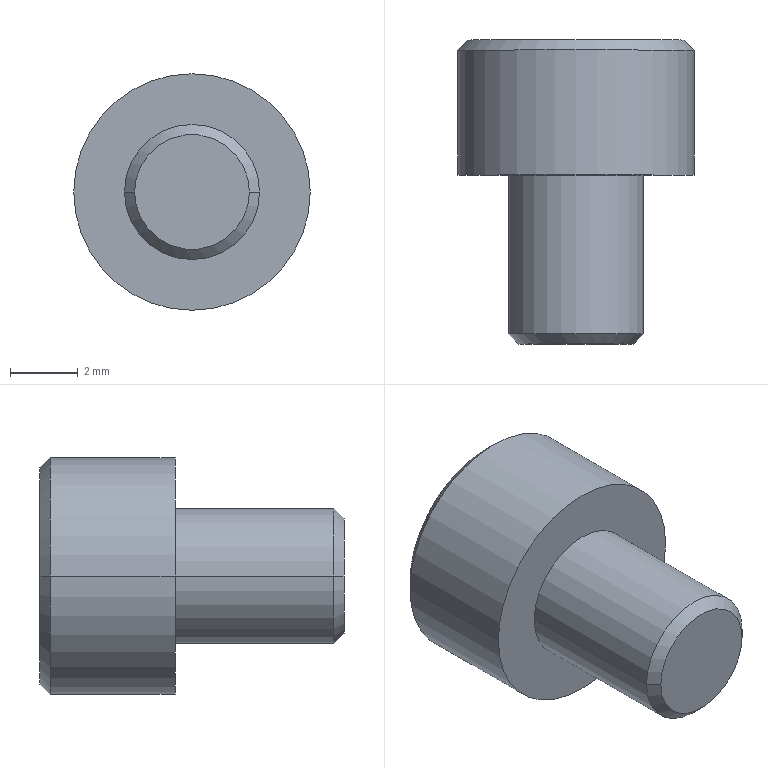Part | NX | 1 solid | 55 faces | box 7 x 9 x 7 mm | volume 197.52 mm3 | plane 45 | cone 6 | cylinder 4 | commonest cylinder face diameters 4 x2 7 x2
STEP:
#1=CARTESIAN_POINT('',(1.7,-5.,0.));
#2=VERTEX_POINT('',#1);
#3=CARTESIAN_POINT('',(-1.7,-5.,0.));
#4=VERTEX_POINT('',#3);
#5=CARTESIAN_POINT('',(0.,-5.,0.));
#6=DIRECTION('',(0.,1.,0.));
#7=DIRECTION('',(-1.,0.,0.));
#8=AXIS2_PLACEMENT_3D('',#5,#6,#7);
#9=CIRCLE('',#8,1.7);
#10=EDGE_CURVE('',#2,#4,#9,.T.);
#11=ORIENTED_EDGE('',*,*,#10,.F.);
#12=CARTESIAN_POINT('',(0.,-5.,0.));
#13=DIRECTION('',(0.,1.,0.));
#14=DIRECTION('',(-1.,0.,0.));
#15=AXIS2_PLACEMENT_3D('',#12,#13,#14);
#16=CIRCLE('',#15,1.7);
#17=EDGE_CURVE('',#4,#2,#16,.T.);
#18=ORIENTED_EDGE('',*,*,#17,.F.);
#19=EDGE_LOOP('',(#11,#18));
#20=FACE_BOUND('',#19,.T.);
#21=CARTESIAN_POINT('',(0.,-5.,0.));
#22=DIRECTION('',(0.,-1.,0.));
#23=DIRECTION('',(0.,0.,-1.));
#24=AXIS2_PLACEMENT_3D('',#21,#22,#23);
#25=PLANE('',#24);
#26=ADVANCED_FACE('',(#20),#25,.T.);
#27=CARTESIAN_POINT('',(-2.,-4.7,0.));
#28=VERTEX_POINT('',#27);
#29=CARTESIAN_POINT('',(2.,-4.7,0.));
#30=VERTEX_POINT('',#29);
#31=CARTESIAN_POINT('',(0.,-4.7,0.));
#32=DIRECTION('',(0.,1.,0.));
#33=DIRECTION('',(-1.,0.,0.));
#34=AXIS2_PLACEMENT_3D('',#31,#32,#33);
#35=CIRCLE('',#34,2.);
#36=EDGE_CURVE('',#28,#30,#35,.T.);
#37=ORIENTED_EDGE('',*,*,#36,.F.);
#38=CARTESIAN_POINT('',(-1.85,-4.85,0.));
#39=DIRECTION('',(-0.7071,0.7071,0.));
#40=VECTOR('',#39,1000.);
#41=LINE('',#38,#40);
#42=EDGE_CURVE('',#28,#4,#41,.F.);
#43=ORIENTED_EDGE('',*,*,#42,.T.);
#44=ORIENTED_EDGE('',*,*,#17,.T.);
#45=CARTESIAN_POINT('',(1.85,-4.85,0.));
#46=DIRECTION('',(0.7071,0.7071,0.));
#47=VECTOR('',#46,1000.);
#48=LINE('',#45,#47);
#49=EDGE_CURVE('',#30,#2,#48,.F.);
#50=ORIENTED_EDGE('',*,*,#49,.F.);
#51=EDGE_LOOP('',(#37,#43,#44,#50));
#52=FACE_BOUND('',#51,.T.);
#53=CARTESIAN_POINT('',(0.,-4.85,0.));
#54=DIRECTION('',(0.,1.,0.));
#55=DIRECTION('',(1.,0.,0.));
#56=AXIS2_PLACEMENT_3D('',#53,#54,#55);
#57=CONICAL_SURFACE('',#56,1.85,0.7854);
#58=ADVANCED_FACE('',(#52),#57,.T.);
#59=CARTESIAN_POINT('',(-2.,0.,0.));
#60=VERTEX_POINT('',#59);
#61=CARTESIAN_POINT('',(2.,0.,0.));
#62=VERTEX_POINT('',#61);
#63=CARTESIAN_POINT('',(0.,0.,0.));
#64=DIRECTION('',(0.,-1.,0.));
#65=DIRECTION('',(1.,0.,0.));
#66=AXIS2_PLACEMENT_3D('',#63,#64,#65);
#67=CIRCLE('',#66,2.);
#68=EDGE_CURVE('',#60,#62,#67,.T.);
#69=ORIENTED_EDGE('',*,*,#68,.T.);
#70=CARTESIAN_POINT('',(2.,4.45,0.));
#71=DIRECTION('',(0.,-1.,0.));
#72=VECTOR('',#71,1000.);
#73=LINE('',#70,#72);
#74=EDGE_CURVE('',#62,#30,#73,.T.);
#75=ORIENTED_EDGE('',*,*,#74,.T.);
#76=CARTESIAN_POINT('',(0.,-4.7,0.));
#77=DIRECTION('',(0.,1.,0.));
#78=DIRECTION('',(-1.,0.,0.));
#79=AXIS2_PLACEMENT_3D('',#76,#77,#78);
#80=CIRCLE('',#79,2.);
#81=EDGE_CURVE('',#30,#28,#80,.T.);
#82=ORIENTED_EDGE('',*,*,#81,.T.);
#83=CARTESIAN_POINT('',(-2.,4.45,0.));
#84=DIRECTION('',(0.,-1.,0.));
#85=VECTOR('',#84,1000.);
#86=LINE('',#83,#85);
#87=EDGE_CURVE('',#60,#28,#86,.T.);
#88=ORIENTED_EDGE('',*,*,#87,.F.);
#89=EDGE_LOOP('',(#69,#75,#82,#88));
#90=FACE_BOUND('',#89,.T.);
#91=CARTESIAN_POINT('',(0.,4.45,0.));
#92=DIRECTION('',(0.,-1.,0.));
#93=DIRECTION('',(-1.,0.,0.));
#94=AXIS2_PLACEMENT_3D('',#91,#92,#93);
#95=CYLINDRICAL_SURFACE('',#94,2.);
#96=ADVANCED_FACE('',(#90),#95,.T.);
#97=CARTESIAN_POINT('',(0.6667,4.,2.274));
#98=VERTEX_POINT('',#97);
#99=CARTESIAN_POINT('',(0.6667,4.,1.87));
#100=VERTEX_POINT('',#99);
#101=CARTESIAN_POINT('',(0.6667,4.,2.274));
#102=DIRECTION('',(0.,0.,-1.));
#103=VECTOR('',#102,1000.);
#104=LINE('',#101,#103);
#105=EDGE_CURVE('',#98,#100,#104,.T.);
#106=ORIENTED_EDGE('',*,*,#105,.F.);
#107=CARTESIAN_POINT('',(0.6667,3.95,2.274));
#108=VERTEX_POINT('',#107);
#109=CARTESIAN_POINT('',(0.6667,3.95,2.274));
#110=DIRECTION('',(0.,1.,0.));
#111=VECTOR('',#110,1000.);
#112=LINE('',#109,#111);
#113=EDGE_CURVE('',#108,#98,#112,.T.);
#114=ORIENTED_EDGE('',*,*,#113,.F.);
#115=CARTESIAN_POINT('',(0.6667,3.95,1.87));
#116=VERTEX_POINT('',#115);
#117=CARTESIAN_POINT('',(0.6667,3.95,2.274));
#118=DIRECTION('',(0.,0.,-1.));
#119=VECTOR('',#118,1000.);
#120=LINE('',#117,#119);
#121=EDGE_CURVE('',#108,#116,#120,.T.);
#122=ORIENTED_EDGE('',*,*,#121,.T.);
#123=CARTESIAN_POINT('',(0.6667,3.95,1.87));
#124=DIRECTION('',(0.,1.,0.));
#125=VECTOR('',#124,1000.);
#126=LINE('',#123,#125);
#127=EDGE_CURVE('',#116,#100,#126,.T.);
#128=ORIENTED_EDGE('',*,*,#127,.T.);
#129=EDGE_LOOP('',(#106,#114,#122,#128));
#130=FACE_BOUND('',#129,.T.);
#131=CARTESIAN_POINT('',(0.6667,4.,1.87));
#132=DIRECTION('',(-1.,0.,0.));
#133=DIRECTION('',(0.,0.,1.));
#134=AXIS2_PLACEMENT_3D('',#131,#132,#133);
#135=PLANE('',#134);
#136=ADVANCED_FACE('',(#130),#135,.F.);
#137=CARTESIAN_POINT('',(0.3125,4.,2.274));
#138=VERTEX_POINT('',#137);
#139=CARTESIAN_POINT('',(0.3125,4.,2.274));
#140=DIRECTION('',(0.659,0.,-0.7522));
#141=VECTOR('',#140,1000.);
#142=LINE('',#139,#141);
#143=EDGE_CURVE('',#138,#100,#142,.T.);
#144=ORIENTED_EDGE('',*,*,#143,.T.);
#145=ORIENTED_EDGE('',*,*,#127,.F.);
#146=CARTESIAN_POINT('',(0.3125,3.95,2.274));
#147=VERTEX_POINT('',#146);
#148=CARTESIAN_POINT('',(0.6667,3.95,1.87));
#149=DIRECTION('',(-0.659,0.,0.7522));
#150=VECTOR('',#149,1000.);
#151=LINE('',#148,#150);
#152=EDGE_CURVE('',#116,#147,#151,.T.);
#153=ORIENTED_EDGE('',*,*,#152,.T.);
#154=CARTESIAN_POINT('',(0.3125,3.95,2.274));
#155=DIRECTION('',(0.,1.,0.));
#156=VECTOR('',#155,1000.);
#157=LINE('',#154,#156);
#158=EDGE_CURVE('',#147,#138,#157,.T.);
#159=ORIENTED_EDGE('',*,*,#158,.T.);
#160=EDGE_LOOP('',(#144,#145,#153,#159));
#161=FACE_BOUND('',#160,.T.);
#162=CARTESIAN_POINT('',(0.3125,4.,2.274));
#163=DIRECTION('',(0.7522,0.,0.659));
#164=DIRECTION('',(0.,-1.,0.));
#165=AXIS2_PLACEMENT_3D('',#162,#163,#164);
#166=PLANE('',#165);
#167=ADVANCED_FACE('',(#161),#166,.F.);
#168=CARTESIAN_POINT('',(-3.5,0.,0.));
#169=VERTEX_POINT('',#168);
#170=CARTESIAN_POINT('',(3.5,0.,0.));
#171=VERTEX_POINT('',#170);
#172=CARTESIAN_POINT('',(0.,0.,0.));
#173=DIRECTION('',(0.,1.,0.));
#174=DIRECTION('',(-1.,0.,0.));
#175=AXIS2_PLACEMENT_3D('',#172,#173,#174);
#176=CIRCLE('',#175,3.5);
#177=EDGE_CURVE('',#169,#171,#176,.T.);
#178=ORIENTED_EDGE('',*,*,#177,.F.);
#179=CARTESIAN_POINT('',(0.,0.,0.));
#180=DIRECTION('',(0.,1.,0.));
#181=DIRECTION('',(-1.,0.,0.));
#182=AXIS2_PLACEMENT_3D('',#179,#180,#181);
#183=CIRCLE('',#182,3.5);
#184=EDGE_CURVE('',#171,#169,#183,.T.);
#185=ORIENTED_EDGE('',*,*,#184,.F.);
#186=EDGE_LOOP('',(#178,#185));
#187=FACE_BOUND('',#186,.T.);
#188=ORIENTED_EDGE('',*,*,#68,.F.);
#189=CARTESIAN_POINT('',(0.,0.,0.));
#190=DIRECTION('',(0.,-1.,0.));
#191=DIRECTION('',(1.,0.,0.));
#192=AXIS2_PLACEMENT_3D('',#189,#190,#191);
#193=CIRCLE('',#192,2.);
#194=EDGE_CURVE('',#62,#60,#193,.T.);
#195=ORIENTED_EDGE('',*,*,#194,.F.);
#196=EDGE_LOOP('',(#188,#195));
#197=FACE_BOUND('',#196,.T.);
#198=CARTESIAN_POINT('',(0.,0.,0.));
#199=DIRECTION('',(0.,-1.,0.));
#200=DIRECTION('',(0.,0.,-1.));
#201=AXIS2_PLACEMENT_3D('',#198,#199,#200);
#202=PLANE('',#201);
#203=ADVANCED_FACE('',(#187,#197),#202,.T.);
#204=ORIENTED_EDGE('',*,*,#177,.T.);
#205=CARTESIAN_POINT('',(3.5,3.7,0.));
#206=VERTEX_POINT('',#205);
#207=CARTESIAN_POINT('',(3.5,4.45,0.));
#208=DIRECTION('',(0.,-1.,0.));
#209=VECTOR('',#208,1000.);
#210=LINE('',#207,#209);
#211=EDGE_CURVE('',#206,#171,#210,.T.);
#212=ORIENTED_EDGE('',*,*,#211,.F.);
#213=CARTESIAN_POINT('',(-3.5,3.7,0.));
#214=VERTEX_POINT('',#213);
#215=CARTESIAN_POINT('',(0.,3.7,0.));
#216=DIRECTION('',(0.,-1.,0.));
#217=DIRECTION('',(1.,0.,0.));
#218=AXIS2_PLACEMENT_3D('',#215,#216,#217);
#219=CIRCLE('',#218,3.5);
#220=EDGE_CURVE('',#206,#214,#219,.T.);
#221=ORIENTED_EDGE('',*,*,#220,.T.);
#222=CARTESIAN_POINT('',(-3.5,4.45,0.));
#223=DIRECTION('',(0.,-1.,0.));
#224=VECTOR('',#223,1000.);
#225=LINE('',#222,#224);
#226=EDGE_CURVE('',#214,#169,#225,.T.);
#227=ORIENTED_EDGE('',*,*,#226,.T.);
#228=EDGE_LOOP('',(#204,#212,#221,#227));
#229=FACE_BOUND('',#228,.T.);
#230=CARTESIAN_POINT('',(0.,4.45,0.));
#231=DIRECTION('',(0.,-1.,0.));
#232=DIRECTION('',(-1.,0.,0.));
#233=AXIS2_PLACEMENT_3D('',#230,#231,#232);
#234=CYLINDRICAL_SURFACE('',#233,3.5);
#235=ADVANCED_FACE('',(#229),#234,.T.);
#236=CARTESIAN_POINT('',(0.1667,3.95,2.274));
#237=VERTEX_POINT('',#236);
#238=CARTESIAN_POINT('',(0.6667,3.95,1.7));
#239=VERTEX_POINT('',#238);
#240=CARTESIAN_POINT('',(0.1667,3.95,2.274));
#241=DIRECTION('',(0.6565,0.,-0.7543));
#242=VECTOR('',#241,1000.);
#243=LINE('',#240,#242);
#244=EDGE_CURVE('',#237,#239,#243,.T.);
#245=ORIENTED_EDGE('',*,*,#244,.F.);
#246=CARTESIAN_POINT('',(0.1667,3.95,2.402));
#247=VERTEX_POINT('',#246);
#248=CARTESIAN_POINT('',(0.1667,3.95,2.402));
#249=DIRECTION('',(0.,0.,-1.));
#250=VECTOR('',#249,1000.);
#251=LINE('',#248,#250);
#252=EDGE_CURVE('',#247,#237,#251,.T.);
#253=ORIENTED_EDGE('',*,*,#252,.F.);
#254=CARTESIAN_POINT('',(0.6667,3.95,2.402));
#255=VERTEX_POINT('',#254);
#256=CARTESIAN_POINT('',(0.6667,3.95,2.402));
#257=DIRECTION('',(-1.,0.,0.));
#258=VECTOR('',#257,1000.);
#259=LINE('',#256,#258);
#260=EDGE_CURVE('',#255,#247,#259,.T.);
#261=ORIENTED_EDGE('',*,*,#260,.F.);
#262=CARTESIAN_POINT('',(0.6667,3.95,2.7));
#263=VERTEX_POINT('',#262);
#264=CARTESIAN_POINT('',(0.6667,3.95,2.7));
#265=DIRECTION('',(0.,0.,-1.));
#266=VECTOR('',#265,1000.);
#267=LINE('',#264,#266);
#268=EDGE_CURVE('',#263,#255,#267,.T.);
#269=ORIENTED_EDGE('',*,*,#268,.F.);
#270=CARTESIAN_POINT('',(0.7917,3.95,2.7));
#271=VERTEX_POINT('',#270);
#272=CARTESIAN_POINT('',(0.7917,3.95,2.7));
#273=DIRECTION('',(-1.,0.,0.));
#274=VECTOR('',#273,1000.);
#275=LINE('',#272,#274);
#276=EDGE_CURVE('',#271,#263,#275,.T.);
#277=ORIENTED_EDGE('',*,*,#276,.F.);
#278=CARTESIAN_POINT('',(0.7917,3.95,2.402));
#279=VERTEX_POINT('',#278);
#280=CARTESIAN_POINT('',(0.7917,3.95,2.402));
#281=DIRECTION('',(0.,0.,1.));
#282=VECTOR('',#281,1000.);
#283=LINE('',#280,#282);
#284=EDGE_CURVE('',#279,#271,#283,.T.);
#285=ORIENTED_EDGE('',*,*,#284,.F.);
#286=CARTESIAN_POINT('',(1.,3.95,2.402));
#287=VERTEX_POINT('',#286);
#288=CARTESIAN_POINT('',(1.,3.95,2.402));
#289=DIRECTION('',(-1.,0.,0.));
#290=VECTOR('',#289,1000.);
#291=LINE('',#288,#290);
#292=EDGE_CURVE('',#287,#279,#291,.T.);
#293=ORIENTED_EDGE('',*,*,#292,.F.);
#294=CARTESIAN_POINT('',(1.,3.95,2.274));
#295=VERTEX_POINT('',#294);
#296=CARTESIAN_POINT('',(1.,3.95,2.274));
#297=DIRECTION('',(0.,0.,1.));
#298=VECTOR('',#297,1000.);
#299=LINE('',#296,#298);
#300=EDGE_CURVE('',#295,#287,#299,.T.);
#301=ORIENTED_EDGE('',*,*,#300,.F.);
#302=CARTESIAN_POINT('',(0.7917,3.95,2.274));
#303=VERTEX_POINT('',#302);
#304=CARTESIAN_POINT('',(0.7917,3.95,2.274));
#305=DIRECTION('',(1.,0.,0.));
#306=VECTOR('',#305,1000.);
#307=LINE('',#304,#306);
#308=EDGE_CURVE('',#303,#295,#307,.T.);
#309=ORIENTED_EDGE('',*,*,#308,.F.);
#310=CARTESIAN_POINT('',(0.7917,3.95,1.7));
#311=VERTEX_POINT('',#310);
#312=CARTESIAN_POINT('',(0.7917,3.95,1.7));
#313=DIRECTION('',(0.,0.,1.));
#314=VECTOR('',#313,1000.);
#315=LINE('',#312,#314);
#316=EDGE_CURVE('',#311,#303,#315,.T.);
#317=ORIENTED_EDGE('',*,*,#316,.F.);
#318=CARTESIAN_POINT('',(0.6667,3.95,1.7));
#319=DIRECTION('',(1.,0.,0.));
#320=VECTOR('',#319,1000.);
#321=LINE('',#318,#320);
#322=EDGE_CURVE('',#239,#311,#321,.T.);
#323=ORIENTED_EDGE('',*,*,#322,.F.);
#324=EDGE_LOOP('',(#245,#253,#261,#269,#277,#285,#293,#301,#309,#317,#323));
#325=FACE_BOUND('',#324,.T.);
#326=ORIENTED_EDGE('',*,*,#152,.F.);
#327=ORIENTED_EDGE('',*,*,#121,.F.);
#328=CARTESIAN_POINT('',(0.3125,3.95,2.274));
#329=DIRECTION('',(1.,0.,0.));
#330=VECTOR('',#329,1000.);
#331=LINE('',#328,#330);
#332=EDGE_CURVE('',#147,#108,#331,.T.);
#333=ORIENTED_EDGE('',*,*,#332,.F.);
#334=EDGE_LOOP('',(#326,#327,#333));
#335=FACE_BOUND('',#334,.T.);
#336=CARTESIAN_POINT('',(0.,3.95,0.));
#337=DIRECTION('',(0.,1.,0.));
#338=DIRECTION('',(1.,0.,0.));
#339=AXIS2_PLACEMENT_3D('',#336,#337,#338);
#340=PLANE('',#339);
#341=ADVANCED_FACE('',(#325,#335),#340,.T.);
#342=CARTESIAN_POINT('',(0.,3.7,0.));
#343=DIRECTION('',(0.,-1.,0.));
#344=DIRECTION('',(1.,0.,0.));
#345=AXIS2_PLACEMENT_3D('',#342,#343,#344);
#346=CIRCLE('',#345,3.5);
#347=EDGE_CURVE('',#214,#206,#346,.T.);
#348=ORIENTED_EDGE('',*,*,#347,.F.);
#349=CARTESIAN_POINT('',(-3.2,4.,0.));
#350=VERTEX_POINT('',#349);
#351=CARTESIAN_POINT('',(-3.35,3.85,0.));
#352=DIRECTION('',(-0.7071,-0.7071,0.));
#353=VECTOR('',#352,1000.);
#354=LINE('',#351,#353);
#355=EDGE_CURVE('',#214,#350,#354,.F.);
#356=ORIENTED_EDGE('',*,*,#355,.T.);
#357=CARTESIAN_POINT('',(3.2,4.,0.));
#358=VERTEX_POINT('',#357);
#359=CARTESIAN_POINT('',(0.,4.,0.));
#360=DIRECTION('',(0.,-1.,0.));
#361=DIRECTION('',(-1.,0.,0.));
#362=AXIS2_PLACEMENT_3D('',#359,#360,#361);
#363=CIRCLE('',#362,3.2);
#364=EDGE_CURVE('',#350,#358,#363,.T.);
#365=ORIENTED_EDGE('',*,*,#364,.T.);
#366=CARTESIAN_POINT('',(3.35,3.85,0.));
#367=DIRECTION('',(0.7071,-0.7071,0.));
#368=VECTOR('',#367,1000.);
#369=LINE('',#366,#368);
#370=EDGE_CURVE('',#206,#358,#369,.F.);
#371=ORIENTED_EDGE('',*,*,#370,.F.);
#372=EDGE_LOOP('',(#348,#356,#365,#371));
#373=FACE_BOUND('',#372,.T.);
#374=CARTESIAN_POINT('',(0.,3.85,0.));
#375=DIRECTION('',(0.,-1.,0.));
#376=DIRECTION('',(-1.,0.,0.));
#377=AXIS2_PLACEMENT_3D('',#374,#375,#376);
#378=CONICAL_SURFACE('',#377,3.35,0.7854);
#379=ADVANCED_FACE('',(#373),#378,.T.);
#380=ORIENTED_EDGE('',*,*,#364,.F.);
#381=CARTESIAN_POINT('',(0.,4.,0.));
#382=DIRECTION('',(0.,-1.,0.));
#383=DIRECTION('',(-1.,0.,0.));
#384=AXIS2_PLACEMENT_3D('',#381,#382,#383);
#385=CIRCLE('',#384,3.2);
#386=EDGE_CURVE('',#358,#350,#385,.T.);
#387=ORIENTED_EDGE('',*,*,#386,.F.);
#388=EDGE_LOOP('',(#380,#387));
#389=FACE_BOUND('',#388,.T.);
#390=CARTESIAN_POINT('',(-0.125,4.,2.7));
#391=VERTEX_POINT('',#390);
#392=CARTESIAN_POINT('',(-0.125,4.,1.913));
#393=VERTEX_POINT('',#392);
#394=CARTESIAN_POINT('',(-0.125,4.,2.7));
#395=DIRECTION('',(0.,0.,-1.));
#396=VECTOR('',#395,1000.);
#397=LINE('',#394,#396);
#398=EDGE_CURVE('',#391,#393,#397,.T.);
#399=ORIENTED_EDGE('',*,*,#398,.T.);
#400=CARTESIAN_POINT('',(-0.4167,4.,2.7));
#401=VERTEX_POINT('',#400);
#402=CARTESIAN_POINT('',(-0.4167,4.,2.7));
#403=DIRECTION('',(0.3474,0.,-0.9377));
#404=VECTOR('',#403,1000.);
#405=LINE('',#402,#404);
#406=EDGE_CURVE('',#401,#393,#405,.T.);
#407=ORIENTED_EDGE('',*,*,#406,.F.);
#408=CARTESIAN_POINT('',(-0.5833,4.,2.7));
#409=VERTEX_POINT('',#408);
#410=CARTESIAN_POINT('',(-0.4167,4.,2.7));
#411=DIRECTION('',(-1.,0.,0.));
#412=VECTOR('',#411,1000.);
#413=LINE('',#410,#412);
#414=EDGE_CURVE('',#401,#409,#413,.T.);
#415=ORIENTED_EDGE('',*,*,#414,.T.);
#416=CARTESIAN_POINT('',(-0.875,4.,1.913));
#417=VERTEX_POINT('',#416);
#418=CARTESIAN_POINT('',(-0.875,4.,1.913));
#419=DIRECTION('',(0.3474,0.,0.9377));
#420=VECTOR('',#419,1000.);
#421=LINE('',#418,#420);
#422=EDGE_CURVE('',#417,#409,#421,.T.);
#423=ORIENTED_EDGE('',*,*,#422,.F.);
#424=CARTESIAN_POINT('',(-0.875,4.,2.7));
#425=VERTEX_POINT('',#424);
#426=CARTESIAN_POINT('',(-0.875,4.,1.913));
#427=DIRECTION('',(0.,0.,1.));
#428=VECTOR('',#427,1000.);
#429=LINE('',#426,#428);
#430=EDGE_CURVE('',#417,#425,#429,.T.);
#431=ORIENTED_EDGE('',*,*,#430,.T.);
#432=CARTESIAN_POINT('',(-1.,4.,2.7));
#433=VERTEX_POINT('',#432);
#434=CARTESIAN_POINT('',(-0.875,4.,2.7));
#435=DIRECTION('',(-1.,0.,0.));
#436=VECTOR('',#435,1000.);
#437=LINE('',#434,#436);
#438=EDGE_CURVE('',#425,#433,#437,.T.);
#439=ORIENTED_EDGE('',*,*,#438,.T.);
#440=CARTESIAN_POINT('',(-1.,4.,1.7));
#441=VERTEX_POINT('',#440);
#442=CARTESIAN_POINT('',(-1.,4.,2.7));
#443=DIRECTION('',(0.,0.,-1.));
#444=VECTOR('',#443,1000.);
#445=LINE('',#442,#444);
#446=EDGE_CURVE('',#433,#441,#445,.T.);
#447=ORIENTED_EDGE('',*,*,#446,.T.);
#448=CARTESIAN_POINT('',(-0.8125,4.,1.7));
#449=VERTEX_POINT('',#448);
#450=CARTESIAN_POINT('',(-1.,4.,1.7));
#451=DIRECTION('',(1.,0.,0.));
#452=VECTOR('',#451,1000.);
#453=LINE('',#450,#452);
#454=EDGE_CURVE('',#441,#449,#453,.T.);
#455=ORIENTED_EDGE('',*,*,#454,.T.);
#456=CARTESIAN_POINT('',(-0.5,4.,2.594));
#457=VERTEX_POINT('',#456);
#458=CARTESIAN_POINT('',(-0.5,4.,2.594));
#459=DIRECTION('',(-0.3301,0.,-0.9439));
#460=VECTOR('',#459,1000.);
#461=LINE('',#458,#460);
#462=EDGE_CURVE('',#457,#449,#461,.T.);
#463=ORIENTED_EDGE('',*,*,#462,.F.);
#464=CARTESIAN_POINT('',(-0.1875,4.,1.7));
#465=VERTEX_POINT('',#464);
#466=CARTESIAN_POINT('',(-0.1875,4.,1.7));
#467=DIRECTION('',(-0.3301,0.,0.9439));
#468=VECTOR('',#467,1000.);
#469=LINE('',#466,#468);
#470=EDGE_CURVE('',#465,#457,#469,.T.);
#471=ORIENTED_EDGE('',*,*,#470,.F.);
#472=CARTESIAN_POINT('',(-0.05551,4.,1.7));
#473=VERTEX_POINT('',#472);
#474=CARTESIAN_POINT('',(-0.1875,4.,1.7));
#475=DIRECTION('',(1.,0.,0.));
#476=VECTOR('',#475,1000.);
#477=LINE('',#474,#476);
#478=EDGE_CURVE('',#465,#473,#477,.T.);
#479=ORIENTED_EDGE('',*,*,#478,.T.);
#480=CARTESIAN_POINT('',(-1.5,4.,0.866));
#481=VERTEX_POINT('',#480);
#482=CARTESIAN_POINT('',(-1.5,4.,0.866));
#483=DIRECTION('',(0.866,0.,0.5));
#484=VECTOR('',#483,1000.);
#485=LINE('',#482,#484);
#486=EDGE_CURVE('',#481,#473,#485,.T.);
#487=ORIENTED_EDGE('',*,*,#486,.F.);
#488=CARTESIAN_POINT('',(-1.5,4.,-0.866));
#489=VERTEX_POINT('',#488);
#490=CARTESIAN_POINT('',(-1.5,4.,0.866));
#491=DIRECTION('',(0.,0.,-1.));
#492=VECTOR('',#491,1000.);
#493=LINE('',#490,#492);
#494=EDGE_CURVE('',#481,#489,#493,.T.);
#495=ORIENTED_EDGE('',*,*,#494,.T.);
#496=CARTESIAN_POINT('',(0.,4.,-1.732));
#497=VERTEX_POINT('',#496);
#498=CARTESIAN_POINT('',(0.,4.,-1.732));
#499=DIRECTION('',(-0.866,0.,0.5));
#500=VECTOR('',#499,1000.);
#501=LINE('',#498,#500);
#502=EDGE_CURVE('',#497,#489,#501,.T.);
#503=ORIENTED_EDGE('',*,*,#502,.F.);
#504=CARTESIAN_POINT('',(1.5,4.,-0.866));
#505=VERTEX_POINT('',#504);
#506=CARTESIAN_POINT('',(1.5,4.,-0.866));
#507=DIRECTION('',(-0.866,0.,-0.5));
#508=VECTOR('',#507,1000.);
#509=LINE('',#506,#508);
#510=EDGE_CURVE('',#505,#497,#509,.T.);
#511=ORIENTED_EDGE('',*,*,#510,.F.);
#512=CARTESIAN_POINT('',(1.5,4.,0.866));
#513=VERTEX_POINT('',#512);
#514=CARTESIAN_POINT('',(1.5,4.,-0.866));
#515=DIRECTION('',(0.,0.,1.));
#516=VECTOR('',#515,1000.);
#517=LINE('',#514,#516);
#518=EDGE_CURVE('',#505,#513,#517,.T.);
#519=ORIENTED_EDGE('',*,*,#518,.T.);
#520=CARTESIAN_POINT('',(0.,4.,1.732));
#521=VERTEX_POINT('',#520);
#522=CARTESIAN_POINT('',(0.,4.,1.732));
#523=DIRECTION('',(0.866,0.,-0.5));
#524=VECTOR('',#523,1000.);
#525=LINE('',#522,#524);
#526=EDGE_CURVE('',#521,#513,#525,.T.);
#527=ORIENTED_EDGE('',*,*,#526,.F.);
#528=CARTESIAN_POINT('',(0.,4.,2.7));
#529=VERTEX_POINT('',#528);
#530=CARTESIAN_POINT('',(0.,4.,1.732));
#531=DIRECTION('',(0.,0.,1.));
#532=VECTOR('',#531,1000.);
#533=LINE('',#530,#532);
#534=EDGE_CURVE('',#521,#529,#533,.T.);
#535=ORIENTED_EDGE('',*,*,#534,.T.);
#536=CARTESIAN_POINT('',(0.,4.,2.7));
#537=DIRECTION('',(-1.,0.,0.));
#538=VECTOR('',#537,1000.);
#539=LINE('',#536,#538);
#540=EDGE_CURVE('',#529,#391,#539,.T.);
#541=ORIENTED_EDGE('',*,*,#540,.T.);
#542=EDGE_LOOP('',(#399,#407,#415,#423,#431,#439,#447,#455,#463,#471,#479,#487,#495,#503,#511,#519,#527,#535,#541));
#543=FACE_BOUND('',#542,.T.);
#544=CARTESIAN_POINT('',(0.6667,4.,1.7));
#545=VERTEX_POINT('',#544);
#546=CARTESIAN_POINT('',(0.1667,4.,2.274));
#547=VERTEX_POINT('',#546);
#548=CARTESIAN_POINT('',(0.6667,4.,1.7));
#549=DIRECTION('',(-0.6565,0.,0.7543));
#550=VECTOR('',#549,1000.);
#551=LINE('',#548,#550);
#552=EDGE_CURVE('',#545,#547,#551,.T.);
#553=ORIENTED_EDGE('',*,*,#552,.F.);
#554=CARTESIAN_POINT('',(0.7917,4.,1.7));
#555=VERTEX_POINT('',#554);
#556=CARTESIAN_POINT('',(0.6667,4.,1.7));
#557=DIRECTION('',(1.,0.,0.));
#558=VECTOR('',#557,1000.);
#559=LINE('',#556,#558);
#560=EDGE_CURVE('',#545,#555,#559,.T.);
#561=ORIENTED_EDGE('',*,*,#560,.T.);
#562=CARTESIAN_POINT('',(0.7917,4.,2.274));
#563=VERTEX_POINT('',#562);
#564=CARTESIAN_POINT('',(0.7917,4.,1.7));
#565=DIRECTION('',(0.,0.,1.));
#566=VECTOR('',#565,1000.);
#567=LINE('',#564,#566);
#568=EDGE_CURVE('',#555,#563,#567,.T.);
#569=ORIENTED_EDGE('',*,*,#568,.T.);
#570=CARTESIAN_POINT('',(1.,4.,2.274));
#571=VERTEX_POINT('',#570);
#572=CARTESIAN_POINT('',(0.7917,4.,2.274));
#573=DIRECTION('',(1.,0.,0.));
#574=VECTOR('',#573,1000.);
#575=LINE('',#572,#574);
#576=EDGE_CURVE('',#563,#571,#575,.T.);
#577=ORIENTED_EDGE('',*,*,#576,.T.);
#578=CARTESIAN_POINT('',(1.,4.,2.402));
#579=VERTEX_POINT('',#578);
#580=CARTESIAN_POINT('',(1.,4.,2.274));
#581=DIRECTION('',(0.,0.,1.));
#582=VECTOR('',#581,1000.);
#583=LINE('',#580,#582);
#584=EDGE_CURVE('',#571,#579,#583,.T.);
#585=ORIENTED_EDGE('',*,*,#584,.T.);
#586=CARTESIAN_POINT('',(0.7917,4.,2.402));
#587=VERTEX_POINT('',#586);
#588=CARTESIAN_POINT('',(1.,4.,2.402));
#589=DIRECTION('',(-1.,0.,0.));
#590=VECTOR('',#589,1000.);
#591=LINE('',#588,#590);
#592=EDGE_CURVE('',#579,#587,#591,.T.);
#593=ORIENTED_EDGE('',*,*,#592,.T.);
#594=CARTESIAN_POINT('',(0.7917,4.,2.7));
#595=VERTEX_POINT('',#594);
#596=CARTESIAN_POINT('',(0.7917,4.,2.402));
#597=DIRECTION('',(0.,0.,1.));
#598=VECTOR('',#597,1000.);
#599=LINE('',#596,#598);
#600=EDGE_CURVE('',#587,#595,#599,.T.);
#601=ORIENTED_EDGE('',*,*,#600,.T.);
#602=CARTESIAN_POINT('',(0.6667,4.,2.7));
#603=VERTEX_POINT('',#602);
#604=CARTESIAN_POINT('',(0.7917,4.,2.7));
#605=DIRECTION('',(-1.,0.,0.));
#606=VECTOR('',#605,1000.);
#607=LINE('',#604,#606);
#608=EDGE_CURVE('',#595,#603,#607,.T.);
#609=ORIENTED_EDGE('',*,*,#608,.T.);
#610=CARTESIAN_POINT('',(0.6667,4.,2.402));
#611=VERTEX_POINT('',#610);
#612=CARTESIAN_POINT('',(0.6667,4.,2.7));
#613=DIRECTION('',(0.,0.,-1.));
#614=VECTOR('',#613,1000.);
#615=LINE('',#612,#614);
#616=EDGE_CURVE('',#603,#611,#615,.T.);
#617=ORIENTED_EDGE('',*,*,#616,.T.);
#618=CARTESIAN_POINT('',(0.1667,4.,2.402));
#619=VERTEX_POINT('',#618);
#620=CARTESIAN_POINT('',(0.6667,4.,2.402));
#621=DIRECTION('',(-1.,0.,0.));
#622=VECTOR('',#621,1000.);
#623=LINE('',#620,#622);
#624=EDGE_CURVE('',#611,#619,#623,.T.);
#625=ORIENTED_EDGE('',*,*,#624,.T.);
#626=CARTESIAN_POINT('',(0.1667,4.,2.402));
#627=DIRECTION('',(0.,0.,-1.));
#628=VECTOR('',#627,1000.);
#629=LINE('',#626,#628);
#630=EDGE_CURVE('',#619,#547,#629,.T.);
#631=ORIENTED_EDGE('',*,*,#630,.T.);
#632=EDGE_LOOP('',(#553,#561,#569,#577,#585,#593,#601,#609,#617,#625,#631));
#633=FACE_BOUND('',#632,.T.);
#634=CARTESIAN_POINT('',(0.,4.,0.));
#635=DIRECTION('',(0.,-1.,0.));
#636=DIRECTION('',(0.,0.,-1.));
#637=AXIS2_PLACEMENT_3D('',#634,#635,#636);
#638=PLANE('',#637);
#639=ADVANCED_FACE('',(#389,#543,#633),#638,.F.);
#640=ORIENTED_EDGE('',*,*,#143,.F.);
#641=CARTESIAN_POINT('',(0.3125,4.,2.274));
#642=DIRECTION('',(1.,0.,0.));
#643=VECTOR('',#642,1000.);
#644=LINE('',#641,#643);
#645=EDGE_CURVE('',#138,#98,#644,.T.);
#646=ORIENTED_EDGE('',*,*,#645,.T.);
#647=ORIENTED_EDGE('',*,*,#105,.T.);
#648=EDGE_LOOP('',(#640,#646,#647));
#649=FACE_BOUND('',#648,.T.);
#650=CARTESIAN_POINT('',(0.,4.,0.));
#651=DIRECTION('',(0.,-1.,0.));
#652=DIRECTION('',(0.,0.,-1.));
#653=AXIS2_PLACEMENT_3D('',#650,#651,#652);
#654=PLANE('',#653);
#655=ADVANCED_FACE('',(#649),#654,.F.);
#656=ORIENTED_EDGE('',*,*,#398,.F.);
#657=CARTESIAN_POINT('',(-0.125,3.95,2.7));
#658=VERTEX_POINT('',#657);
#659=CARTESIAN_POINT('',(-0.125,3.95,2.7));
#660=DIRECTION('',(0.,1.,0.));
#661=VECTOR('',#660,1000.);
#662=LINE('',#659,#661);
#663=EDGE_CURVE('',#658,#391,#662,.T.);
#664=ORIENTED_EDGE('',*,*,#663,.F.);
#665=CARTESIAN_POINT('',(-0.125,3.95,1.913));
#666=VERTEX_POINT('',#665);
#667=CARTESIAN_POINT('',(-0.125,3.95,2.7));
#668=DIRECTION('',(0.,0.,-1.));
#669=VECTOR('',#668,1000.);
#670=LINE('',#667,#669);
#671=EDGE_CURVE('',#658,#666,#670,.T.);
#672=ORIENTED_EDGE('',*,*,#671,.T.);
#673=CARTESIAN_POINT('',(-0.125,3.95,1.913));
#674=DIRECTION('',(0.,1.,0.));
#675=VECTOR('',#674,1000.);
#676=LINE('',#673,#675);
#677=EDGE_CURVE('',#666,#393,#676,.T.);
#678=ORIENTED_EDGE('',*,*,#677,.T.);
#679=EDGE_LOOP('',(#656,#664,#672,#678));
#680=FACE_BOUND('',#679,.T.);
#681=CARTESIAN_POINT('',(-0.125,4.,1.913));
#682=DIRECTION('',(-1.,0.,0.));
#683=DIRECTION('',(0.,0.,1.));
#684=AXIS2_PLACEMENT_3D('',#681,#682,#683);
#685=PLANE('',#684);
#686=ADVANCED_FACE('',(#680),#685,.F.);
#687=ORIENTED_EDGE('',*,*,#406,.T.);
#688=ORIENTED_EDGE('',*,*,#677,.F.);
#689=CARTESIAN_POINT('',(-0.4167,3.95,2.7));
#690=VERTEX_POINT('',#689);
#691=CARTESIAN_POINT('',(-0.125,3.95,1.913));
#692=DIRECTION('',(-0.3474,0.,0.9377));
#693=VECTOR('',#692,1000.);
#694=LINE('',#691,#693);
#695=EDGE_CURVE('',#666,#690,#694,.T.);
#696=ORIENTED_EDGE('',*,*,#695,.T.);
#697=CARTESIAN_POINT('',(-0.4167,3.95,2.7));
#698=DIRECTION('',(0.,1.,0.));
#699=VECTOR('',#698,1000.);
#700=LINE('',#697,#699);
#701=EDGE_CURVE('',#690,#401,#700,.T.);
#702=ORIENTED_EDGE('',*,*,#701,.T.);
#703=EDGE_LOOP('',(#687,#688,#696,#702));
#704=FACE_BOUND('',#703,.T.);
#705=CARTESIAN_POINT('',(-0.4167,4.,2.7));
#706=DIRECTION('',(0.9377,0.,0.3474));
#707=DIRECTION('',(0.,-1.,0.));
#708=AXIS2_PLACEMENT_3D('',#705,#706,#707);
#709=PLANE('',#708);
#710=ADVANCED_FACE('',(#704),#709,.F.);
#711=ORIENTED_EDGE('',*,*,#414,.F.);
#712=ORIENTED_EDGE('',*,*,#701,.F.);
#713=CARTESIAN_POINT('',(-0.5833,3.95,2.7));
#714=VERTEX_POINT('',#713);
#715=CARTESIAN_POINT('',(-0.4167,3.95,2.7));
#716=DIRECTION('',(-1.,0.,0.));
#717=VECTOR('',#716,1000.);
#718=LINE('',#715,#717);
#719=EDGE_CURVE('',#690,#714,#718,.T.);
#720=ORIENTED_EDGE('',*,*,#719,.T.);
#721=CARTESIAN_POINT('',(-0.5833,3.95,2.7));
#722=DIRECTION('',(0.,1.,0.));
#723=VECTOR('',#722,1000.);
#724=LINE('',#721,#723);
#725=EDGE_CURVE('',#714,#409,#724,.T.);
#726=ORIENTED_EDGE('',*,*,#725,.T.);
#727=EDGE_LOOP('',(#711,#712,#720,#726));
#728=FACE_BOUND('',#727,.T.);
#729=CARTESIAN_POINT('',(-0.5833,4.,2.7));
#730=DIRECTION('',(0.,0.,1.));
#731=DIRECTION('',(1.,0.,0.));
#732=AXIS2_PLACEMENT_3D('',#729,#730,#731);
#733=PLANE('',#732);
#734=ADVANCED_FACE('',(#728),#733,.F.);
#735=ORIENTED_EDGE('',*,*,#422,.T.);
#736=ORIENTED_EDGE('',*,*,#725,.F.);
#737=CARTESIAN_POINT('',(-0.875,3.95,1.913));
#738=VERTEX_POINT('',#737);
#739=CARTESIAN_POINT('',(-0.5833,3.95,2.7));
#740=DIRECTION('',(-0.3474,0.,-0.9377));
#741=VECTOR('',#740,1000.);
#742=LINE('',#739,#741);
#743=EDGE_CURVE('',#714,#738,#742,.T.);
#744=ORIENTED_EDGE('',*,*,#743,.T.);
#745=CARTESIAN_POINT('',(-0.875,3.95,1.913));
#746=DIRECTION('',(0.,1.,0.));
#747=VECTOR('',#746,1000.);
#748=LINE('',#745,#747);
#749=EDGE_CURVE('',#738,#417,#748,.T.);
#750=ORIENTED_EDGE('',*,*,#749,.T.);
#751=EDGE_LOOP('',(#735,#736,#744,#750));
#752=FACE_BOUND('',#751,.T.);
#753=CARTESIAN_POINT('',(-0.875,4.,1.913));
#754=DIRECTION('',(-0.9377,0.,0.3474));
#755=DIRECTION('',(0.,1.,0.));
#756=AXIS2_PLACEMENT_3D('',#753,#754,#755);
#757=PLANE('',#756);
#758=ADVANCED_FACE('',(#752),#757,.F.);
#759=ORIENTED_EDGE('',*,*,#430,.F.);
#760=ORIENTED_EDGE('',*,*,#749,.F.);
#761=CARTESIAN_POINT('',(-0.875,3.95,2.7));
#762=VERTEX_POINT('',#761);
#763=CARTESIAN_POINT('',(-0.875,3.95,1.913));
#764=DIRECTION('',(0.,0.,1.));
#765=VECTOR('',#764,1000.);
#766=LINE('',#763,#765);
#767=EDGE_CURVE('',#738,#762,#766,.T.);
#768=ORIENTED_EDGE('',*,*,#767,.T.);
#769=CARTESIAN_POINT('',(-0.875,3.95,2.7));
#770=DIRECTION('',(0.,1.,0.));
#771=VECTOR('',#770,1000.);
#772=LINE('',#769,#771);
#773=EDGE_CURVE('',#762,#425,#772,.T.);
#774=ORIENTED_EDGE('',*,*,#773,.T.);
#775=EDGE_LOOP('',(#759,#760,#768,#774));
#776=FACE_BOUND('',#775,.T.);
#777=CARTESIAN_POINT('',(-0.875,4.,2.7));
#778=DIRECTION('',(1.,0.,0.));
#779=DIRECTION('',(0.,1.,0.));
#780=AXIS2_PLACEMENT_3D('',#777,#778,#779);
#781=PLANE('',#780);
#782=ADVANCED_FACE('',(#776),#781,.F.);
#783=ORIENTED_EDGE('',*,*,#438,.F.);
#784=ORIENTED_EDGE('',*,*,#773,.F.);
#785=CARTESIAN_POINT('',(-1.,3.95,2.7));
#786=VERTEX_POINT('',#785);
#787=CARTESIAN_POINT('',(-0.875,3.95,2.7));
#788=DIRECTION('',(-1.,0.,0.));
#789=VECTOR('',#788,1000.);
#790=LINE('',#787,#789);
#791=EDGE_CURVE('',#762,#786,#790,.T.);
#792=ORIENTED_EDGE('',*,*,#791,.T.);
#793=CARTESIAN_POINT('',(-1.,3.95,2.7));
#794=DIRECTION('',(0.,1.,0.));
#795=VECTOR('',#794,1000.);
#796=LINE('',#793,#795);
#797=EDGE_CURVE('',#786,#433,#796,.T.);
#798=ORIENTED_EDGE('',*,*,#797,.T.);
#799=EDGE_LOOP('',(#783,#784,#792,#798));
#800=FACE_BOUND('',#799,.T.);
#801=CARTESIAN_POINT('',(-1.,4.,2.7));
#802=DIRECTION('',(0.,0.,1.));
#803=DIRECTION('',(1.,0.,0.));
#804=AXIS2_PLACEMENT_3D('',#801,#802,#803);
#805=PLANE('',#804);
#806=ADVANCED_FACE('',(#800),#805,.F.);
#807=ORIENTED_EDGE('',*,*,#446,.F.);
#808=ORIENTED_EDGE('',*,*,#797,.F.);
#809=CARTESIAN_POINT('',(-1.,3.95,1.7));
#810=VERTEX_POINT('',#809);
#811=CARTESIAN_POINT('',(-1.,3.95,2.7));
#812=DIRECTION('',(0.,0.,-1.));
#813=VECTOR('',#812,1000.);
#814=LINE('',#811,#813);
#815=EDGE_CURVE('',#786,#810,#814,.T.);
#816=ORIENTED_EDGE('',*,*,#815,.T.);
#817=CARTESIAN_POINT('',(-1.,3.95,1.7));
#818=DIRECTION('',(0.,1.,0.));
#819=VECTOR('',#818,1000.);
#820=LINE('',#817,#819);
#821=EDGE_CURVE('',#810,#441,#820,.T.);
#822=ORIENTED_EDGE('',*,*,#821,.T.);
#823=EDGE_LOOP('',(#807,#808,#816,#822));
#824=FACE_BOUND('',#823,.T.);
#825=CARTESIAN_POINT('',(-1.,4.,1.7));
#826=DIRECTION('',(-1.,0.,0.));
#827=DIRECTION('',(0.,0.,1.));
#828=AXIS2_PLACEMENT_3D('',#825,#826,#827);
#829=PLANE('',#828);
#830=ADVANCED_FACE('',(#824),#829,.F.);
#831=ORIENTED_EDGE('',*,*,#454,.F.);
#832=ORIENTED_EDGE('',*,*,#821,.F.);
#833=CARTESIAN_POINT('',(-0.8125,3.95,1.7));
#834=VERTEX_POINT('',#833);
#835=CARTESIAN_POINT('',(-1.,3.95,1.7));
#836=DIRECTION('',(1.,0.,0.));
#837=VECTOR('',#836,1000.);
#838=LINE('',#835,#837);
#839=EDGE_CURVE('',#810,#834,#838,.T.);
#840=ORIENTED_EDGE('',*,*,#839,.T.);
#841=CARTESIAN_POINT('',(-0.8125,3.95,1.7));
#842=DIRECTION('',(0.,1.,0.));
#843=VECTOR('',#842,1000.);
#844=LINE('',#841,#843);
#845=EDGE_CURVE('',#834,#449,#844,.T.);
#846=ORIENTED_EDGE('',*,*,#845,.T.);
#847=EDGE_LOOP('',(#831,#832,#840,#846));
#848=FACE_BOUND('',#847,.T.);
#849=CARTESIAN_POINT('',(-0.8125,4.,1.7));
#850=DIRECTION('',(0.,0.,-1.));
#851=DIRECTION('',(0.,-1.,0.));
#852=AXIS2_PLACEMENT_3D('',#849,#850,#851);
#853=PLANE('',#852);
#854=ADVANCED_FACE('',(#848),#853,.F.);
#855=ORIENTED_EDGE('',*,*,#462,.T.);
#856=ORIENTED_EDGE('',*,*,#845,.F.);
#857=CARTESIAN_POINT('',(-0.5,3.95,2.594));
#858=VERTEX_POINT('',#857);
#859=CARTESIAN_POINT('',(-0.8125,3.95,1.7));
#860=DIRECTION('',(0.3301,0.,0.9439));
#861=VECTOR('',#860,1000.);
#862=LINE('',#859,#861);
#863=EDGE_CURVE('',#834,#858,#862,.T.);
#864=ORIENTED_EDGE('',*,*,#863,.T.);
#865=CARTESIAN_POINT('',(-0.5,3.95,2.594));
#866=DIRECTION('',(0.,1.,0.));
#867=VECTOR('',#866,1000.);
#868=LINE('',#865,#867);
#869=EDGE_CURVE('',#858,#457,#868,.T.);
#870=ORIENTED_EDGE('',*,*,#869,.T.);
#871=EDGE_LOOP('',(#855,#856,#864,#870));
#872=FACE_BOUND('',#871,.T.);
#873=CARTESIAN_POINT('',(-0.5,4.,2.594));
#874=DIRECTION('',(0.9439,0.,-0.3301));
#875=DIRECTION('',(0.,-1.,0.));
#876=AXIS2_PLACEMENT_3D('',#873,#874,#875);
#877=PLANE('',#876);
#878=ADVANCED_FACE('',(#872),#877,.F.);
#879=ORIENTED_EDGE('',*,*,#470,.T.);
#880=ORIENTED_EDGE('',*,*,#869,.F.);
#881=CARTESIAN_POINT('',(-0.1875,3.95,1.7));
#882=VERTEX_POINT('',#881);
#883=CARTESIAN_POINT('',(-0.5,3.95,2.594));
#884=DIRECTION('',(0.3301,0.,-0.9439));
#885=VECTOR('',#884,1000.);
#886=LINE('',#883,#885);
#887=EDGE_CURVE('',#858,#882,#886,.T.);
#888=ORIENTED_EDGE('',*,*,#887,.T.);
#889=CARTESIAN_POINT('',(-0.1875,3.95,1.7));
#890=DIRECTION('',(0.,1.,0.));
#891=VECTOR('',#890,1000.);
#892=LINE('',#889,#891);
#893=EDGE_CURVE('',#882,#465,#892,.T.);
#894=ORIENTED_EDGE('',*,*,#893,.T.);
#895=EDGE_LOOP('',(#879,#880,#888,#894));
#896=FACE_BOUND('',#895,.T.);
#897=CARTESIAN_POINT('',(-0.1875,4.,1.7));
#898=DIRECTION('',(-0.9439,0.,-0.3301));
#899=DIRECTION('',(-0.3301,0.,0.9439));
#900=AXIS2_PLACEMENT_3D('',#897,#898,#899);
#901=PLANE('',#900);
#902=ADVANCED_FACE('',(#896),#901,.F.);
#903=ORIENTED_EDGE('',*,*,#478,.F.);
#904=ORIENTED_EDGE('',*,*,#893,.F.);
#905=CARTESIAN_POINT('',(-0.05551,3.95,1.7));
#906=VERTEX_POINT('',#905);
#907=CARTESIAN_POINT('',(-0.1875,3.95,1.7));
#908=DIRECTION('',(1.,0.,0.));
#909=VECTOR('',#908,1000.);
#910=LINE('',#907,#909);
#911=EDGE_CURVE('',#882,#906,#910,.T.);
#912=ORIENTED_EDGE('',*,*,#911,.T.);
#913=CARTESIAN_POINT('',(-0.05551,3.95,1.7));
#914=DIRECTION('',(0.,1.,0.));
#915=VECTOR('',#914,1000.);
#916=LINE('',#913,#915);
#917=EDGE_CURVE('',#906,#473,#916,.T.);
#918=ORIENTED_EDGE('',*,*,#917,.T.);
#919=EDGE_LOOP('',(#903,#904,#912,#918));
#920=FACE_BOUND('',#919,.T.);
#921=CARTESIAN_POINT('',(0.,4.,1.7));
#922=DIRECTION('',(0.,0.,-1.));
#923=DIRECTION('',(0.,-1.,0.));
#924=AXIS2_PLACEMENT_3D('',#921,#922,#923);
#925=PLANE('',#924);
#926=ADVANCED_FACE('',(#920),#925,.F.);
#927=CARTESIAN_POINT('',(0.,3.95,1.732));
#928=VERTEX_POINT('',#927);
#929=CARTESIAN_POINT('',(-0.05551,3.95,1.7));
#930=DIRECTION('',(0.866,0.,0.5));
#931=VECTOR('',#930,1000.);
#932=LINE('',#929,#931);
#933=EDGE_CURVE('',#906,#928,#932,.T.);
#934=ORIENTED_EDGE('',*,*,#933,.T.);
#935=CARTESIAN_POINT('',(0.,2.,1.732));
#936=VERTEX_POINT('',#935);
#937=CARTESIAN_POINT('',(0.,2.,1.732));
#938=DIRECTION('',(0.,1.,0.));
#939=VECTOR('',#938,1000.);
#940=LINE('',#937,#939);
#941=EDGE_CURVE('',#936,#928,#940,.T.);
#942=ORIENTED_EDGE('',*,*,#941,.F.);
#943=CARTESIAN_POINT('',(-0.75,2.,1.299));
#944=VERTEX_POINT('',#943);
#945=CARTESIAN_POINT('',(0.,2.,1.732));
#946=DIRECTION('',(-0.866,0.,-0.5));
#947=VECTOR('',#946,1000.);
#948=LINE('',#945,#947);
#949=EDGE_CURVE('',#936,#944,#948,.T.);
#950=ORIENTED_EDGE('',*,*,#949,.T.);
#951=CARTESIAN_POINT('',(-1.5,2.,0.866));
#952=VERTEX_POINT('',#951);
#953=CARTESIAN_POINT('',(-0.75,2.,1.299));
#954=DIRECTION('',(-0.866,0.,-0.5));
#955=VECTOR('',#954,1000.);
#956=LINE('',#953,#955);
#957=EDGE_CURVE('',#944,#952,#956,.T.);
#958=ORIENTED_EDGE('',*,*,#957,.T.);
#959=CARTESIAN_POINT('',(-1.5,2.,0.866));
#960=DIRECTION('',(0.,1.,0.));
#961=VECTOR('',#960,1000.);
#962=LINE('',#959,#961);
#963=EDGE_CURVE('',#952,#481,#962,.T.);
#964=ORIENTED_EDGE('',*,*,#963,.T.);
#965=ORIENTED_EDGE('',*,*,#486,.T.);
#966=ORIENTED_EDGE('',*,*,#917,.F.);
#967=EDGE_LOOP('',(#934,#942,#950,#958,#964,#965,#966));
#968=FACE_BOUND('',#967,.T.);
#969=CARTESIAN_POINT('',(-1.5,4.,0.866));
#970=DIRECTION('',(-0.5,0.,0.866));
#971=DIRECTION('',(0.,1.,0.));
#972=AXIS2_PLACEMENT_3D('',#969,#970,#971);
#973=PLANE('',#972);
#974=ADVANCED_FACE('',(#968),#973,.F.);
#975=ORIENTED_EDGE('',*,*,#933,.F.);
#976=ORIENTED_EDGE('',*,*,#911,.F.);
#977=ORIENTED_EDGE('',*,*,#887,.F.);
#978=ORIENTED_EDGE('',*,*,#863,.F.);
#979=ORIENTED_EDGE('',*,*,#839,.F.);
#980=ORIENTED_EDGE('',*,*,#815,.F.);
#981=ORIENTED_EDGE('',*,*,#791,.F.);
#982=ORIENTED_EDGE('',*,*,#767,.F.);
#983=ORIENTED_EDGE('',*,*,#743,.F.);
#984=ORIENTED_EDGE('',*,*,#719,.F.);
#985=ORIENTED_EDGE('',*,*,#695,.F.);
#986=ORIENTED_EDGE('',*,*,#671,.F.);
#987=CARTESIAN_POINT('',(0.,3.95,2.7));
#988=VERTEX_POINT('',#987);
#989=CARTESIAN_POINT('',(0.,3.95,2.7));
#990=DIRECTION('',(-1.,0.,0.));
#991=VECTOR('',#990,1000.);
#992=LINE('',#989,#991);
#993=EDGE_CURVE('',#988,#658,#992,.T.);
#994=ORIENTED_EDGE('',*,*,#993,.F.);
#995=CARTESIAN_POINT('',(0.,3.95,1.732));
#996=DIRECTION('',(0.,0.,1.));
#997=VECTOR('',#996,1000.);
#998=LINE('',#995,#997);
#999=EDGE_CURVE('',#928,#988,#998,.T.);
#1000=ORIENTED_EDGE('',*,*,#999,.F.);
#1001=EDGE_LOOP('',(#975,#976,#977,#978,#979,#980,#981,#982,#983,#984,#985,#986,#994,#1000));
#1002=FACE_BOUND('',#1001,.T.);
#1003=CARTESIAN_POINT('',(0.,3.95,0.));
#1004=DIRECTION('',(0.,1.,0.));
#1005=DIRECTION('',(1.,0.,0.));
#1006=AXIS2_PLACEMENT_3D('',#1003,#1004,#1005);
#1007=PLANE('',#1006);
#1008=ADVANCED_FACE('',(#1002),#1007,.T.);
#1009=ORIENTED_EDGE('',*,*,#534,.F.);
#1010=CARTESIAN_POINT('',(0.,3.95,1.732));
#1011=DIRECTION('',(0.,1.,0.));
#1012=VECTOR('',#1011,1000.);
#1013=LINE('',#1010,#1012);
#1014=EDGE_CURVE('',#928,#521,#1013,.T.);
#1015=ORIENTED_EDGE('',*,*,#1014,.F.);
#1016=ORIENTED_EDGE('',*,*,#999,.T.);
#1017=CARTESIAN_POINT('',(0.,3.95,2.7));
#1018=DIRECTION('',(0.,1.,0.));
#1019=VECTOR('',#1018,1000.);
#1020=LINE('',#1017,#1019);
#1021=EDGE_CURVE('',#988,#529,#1020,.T.);
#1022=ORIENTED_EDGE('',*,*,#1021,.T.);
#1023=EDGE_LOOP('',(#1009,#1015,#1016,#1022));
#1024=FACE_BOUND('',#1023,.T.);
#1025=CARTESIAN_POINT('',(0.,4.,2.7));
#1026=DIRECTION('',(1.,0.,0.));
#1027=DIRECTION('',(0.,1.,0.));
#1028=AXIS2_PLACEMENT_3D('',#1025,#1026,#1027);
#1029=PLANE('',#1028);
#1030=ADVANCED_FACE('',(#1024),#1029,.F.);
#1031=ORIENTED_EDGE('',*,*,#540,.F.);
#1032=ORIENTED_EDGE('',*,*,#1021,.F.);
#1033=ORIENTED_EDGE('',*,*,#993,.T.);
#1034=ORIENTED_EDGE('',*,*,#663,.T.);
#1035=EDGE_LOOP('',(#1031,#1032,#1033,#1034));
#1036=FACE_BOUND('',#1035,.T.);
#1037=CARTESIAN_POINT('',(-0.125,4.,2.7));
#1038=DIRECTION('',(0.,0.,1.));
#1039=DIRECTION('',(1.,0.,0.));
#1040=AXIS2_PLACEMENT_3D('',#1037,#1038,#1039);
#1041=PLANE('',#1040);
#1042=ADVANCED_FACE('',(#1036),#1041,.F.);
#1043=ORIENTED_EDGE('',*,*,#1014,.T.);
#1044=ORIENTED_EDGE('',*,*,#526,.T.);
#1045=CARTESIAN_POINT('',(1.5,2.,0.866));
#1046=VERTEX_POINT('',#1045);
#1047=CARTESIAN_POINT('',(1.5,2.,0.866));
#1048=DIRECTION('',(0.,1.,0.));
#1049=VECTOR('',#1048,1000.);
#1050=LINE('',#1047,#1049);
#1051=EDGE_CURVE('',#1046,#513,#1050,.T.);
#1052=ORIENTED_EDGE('',*,*,#1051,.F.);
#1053=CARTESIAN_POINT('',(0.75,2.,1.299));
#1054=VERTEX_POINT('',#1053);
#1055=CARTESIAN_POINT('',(1.5,2.,0.866));
#1056=DIRECTION('',(-0.866,0.,0.5));
#1057=VECTOR('',#1056,1000.);
#1058=LINE('',#1055,#1057);
#1059=EDGE_CURVE('',#1046,#1054,#1058,.T.);
#1060=ORIENTED_EDGE('',*,*,#1059,.T.);
#1061=CARTESIAN_POINT('',(0.75,2.,1.299));
#1062=DIRECTION('',(-0.866,0.,0.5));
#1063=VECTOR('',#1062,1000.);
#1064=LINE('',#1061,#1063);
#1065=EDGE_CURVE('',#1054,#936,#1064,.T.);
#1066=ORIENTED_EDGE('',*,*,#1065,.T.);
#1067=ORIENTED_EDGE('',*,*,#941,.T.);
#1068=EDGE_LOOP('',(#1043,#1044,#1052,#1060,#1066,#1067));
#1069=FACE_BOUND('',#1068,.T.);
#1070=CARTESIAN_POINT('',(0.,4.,1.732));
#1071=DIRECTION('',(0.5,0.,0.866));
#1072=DIRECTION('',(0.,-1.,0.));
#1073=AXIS2_PLACEMENT_3D('',#1070,#1071,#1072);
#1074=PLANE('',#1073);
#1075=ADVANCED_FACE('',(#1069),#1074,.F.);
#1076=CARTESIAN_POINT('',(0.,2.,0.));
#1077=DIRECTION('',(0.,1.,0.));
#1078=DIRECTION('',(-0.5,0.,0.866));
#1079=AXIS2_PLACEMENT_3D('',#1076,#1077,#1078);
#1080=CIRCLE('',#1079,1.5);
#1081=EDGE_CURVE('',#944,#1054,#1080,.T.);
#1082=ORIENTED_EDGE('',*,*,#1081,.F.);
#1083=ORIENTED_EDGE('',*,*,#949,.F.);
#1084=ORIENTED_EDGE('',*,*,#1065,.F.);
#1085=EDGE_LOOP('',(#1082,#1083,#1084));
#1086=FACE_BOUND('',#1085,.T.);
#1087=CARTESIAN_POINT('',(0.,2.,0.));
#1088=DIRECTION('',(0.,1.,0.));
#1089=DIRECTION('',(1.,0.,0.));
#1090=AXIS2_PLACEMENT_3D('',#1087,#1088,#1089);
#1091=PLANE('',#1090);
#1092=ADVANCED_FACE('',(#1086),#1091,.T.);
#1093=CARTESIAN_POINT('',(1.5,2.,0.));
#1094=VERTEX_POINT('',#1093);
#1095=CARTESIAN_POINT('',(0.,2.,0.));
#1096=DIRECTION('',(0.,1.,0.));
#1097=DIRECTION('',(0.5,0.,0.866));
#1098=AXIS2_PLACEMENT_3D('',#1095,#1096,#1097);
#1099=CIRCLE('',#1098,1.5);
#1100=EDGE_CURVE('',#1054,#1094,#1099,.T.);
#1101=ORIENTED_EDGE('',*,*,#1100,.T.);
#1102=CARTESIAN_POINT('',(0.,1.099,0.));
#1103=VERTEX_POINT('',#1102);
#1104=CARTESIAN_POINT('',(0.765,1.558,0.));
#1105=DIRECTION('',(0.8572,0.515,0.));
#1106=VECTOR('',#1105,1000.);
#1107=LINE('',#1104,#1106);
#1108=EDGE_CURVE('',#1094,#1103,#1107,.F.);
#1109=ORIENTED_EDGE('',*,*,#1108,.T.);
#1110=CARTESIAN_POINT('',(-1.5,2.,0.));
#1111=VERTEX_POINT('',#1110);
#1112=CARTESIAN_POINT('',(-0.765,1.558,0.));
#1113=DIRECTION('',(-0.8572,0.515,0.));
#1114=VECTOR('',#1113,1000.);
#1115=LINE('',#1112,#1114);
#1116=EDGE_CURVE('',#1111,#1103,#1115,.F.);
#1117=ORIENTED_EDGE('',*,*,#1116,.F.);
#1118=CARTESIAN_POINT('',(0.,2.,0.));
#1119=DIRECTION('',(0.,1.,0.));
#1120=DIRECTION('',(-1.,0.,0.));
#1121=AXIS2_PLACEMENT_3D('',#1118,#1119,#1120);
#1122=CIRCLE('',#1121,1.5);
#1123=EDGE_CURVE('',#1111,#944,#1122,.T.);
#1124=ORIENTED_EDGE('',*,*,#1123,.T.);
#1125=ORIENTED_EDGE('',*,*,#1081,.T.);
#1126=EDGE_LOOP('',(#1101,#1109,#1117,#1124,#1125));
#1127=FACE_BOUND('',#1126,.T.);
#1128=CARTESIAN_POINT('',(0.,1.558,0.));
#1129=DIRECTION('',(0.,1.,0.));
#1130=DIRECTION('',(1.,0.,0.));
#1131=AXIS2_PLACEMENT_3D('',#1128,#1129,#1130);
#1132=CONICAL_SURFACE('',#1131,0.765,1.03);
#1133=ADVANCED_FACE('',(#1127),#1132,.F.);
#1134=ORIENTED_EDGE('',*,*,#1100,.F.);
#1135=ORIENTED_EDGE('',*,*,#1059,.F.);
#1136=CARTESIAN_POINT('',(1.5,2.,0.));
#1137=DIRECTION('',(0.,0.,1.));
#1138=VECTOR('',#1137,1000.);
#1139=LINE('',#1136,#1138);
#1140=EDGE_CURVE('',#1094,#1046,#1139,.T.);
#1141=ORIENTED_EDGE('',*,*,#1140,.F.);
#1142=EDGE_LOOP('',(#1134,#1135,#1141));
#1143=FACE_BOUND('',#1142,.T.);
#1144=CARTESIAN_POINT('',(0.,2.,0.));
#1145=DIRECTION('',(0.,1.,0.));
#1146=DIRECTION('',(1.,0.,0.));
#1147=AXIS2_PLACEMENT_3D('',#1144,#1145,#1146);
#1148=PLANE('',#1147);
#1149=ADVANCED_FACE('',(#1143),#1148,.T.);
#1150=ORIENTED_EDGE('',*,*,#518,.F.);
#1151=CARTESIAN_POINT('',(1.5,2.,-0.866));
#1152=VERTEX_POINT('',#1151);
#1153=CARTESIAN_POINT('',(1.5,2.,-0.866));
#1154=DIRECTION('',(0.,1.,0.));
#1155=VECTOR('',#1154,1000.);
#1156=LINE('',#1153,#1155);
#1157=EDGE_CURVE('',#1152,#505,#1156,.T.);
#1158=ORIENTED_EDGE('',*,*,#1157,.F.);
#1159=CARTESIAN_POINT('',(1.5,2.,-0.866));
#1160=DIRECTION('',(0.,0.,1.));
#1161=VECTOR('',#1160,1000.);
#1162=LINE('',#1159,#1161);
#1163=EDGE_CURVE('',#1152,#1094,#1162,.T.);
#1164=ORIENTED_EDGE('',*,*,#1163,.T.);
#1165=ORIENTED_EDGE('',*,*,#1140,.T.);
#1166=ORIENTED_EDGE('',*,*,#1051,.T.);
#1167=EDGE_LOOP('',(#1150,#1158,#1164,#1165,#1166));
#1168=FACE_BOUND('',#1167,.T.);
#1169=CARTESIAN_POINT('',(1.5,4.,0.866));
#1170=DIRECTION('',(1.,0.,0.));
#1171=DIRECTION('',(0.,1.,0.));
#1172=AXIS2_PLACEMENT_3D('',#1169,#1170,#1171);
#1173=PLANE('',#1172);
#1174=ADVANCED_FACE('',(#1168),#1173,.F.);
#1175=CARTESIAN_POINT('',(0.75,2.,-1.299));
#1176=VERTEX_POINT('',#1175);
#1177=CARTESIAN_POINT('',(0.,2.,0.));
#1178=DIRECTION('',(0.,1.,0.));
#1179=DIRECTION('',(1.,0.,0.));
#1180=AXIS2_PLACEMENT_3D('',#1177,#1178,#1179);
#1181=CIRCLE('',#1180,1.5);
#1182=EDGE_CURVE('',#1094,#1176,#1181,.T.);
#1183=ORIENTED_EDGE('',*,*,#1182,.F.);
#1184=ORIENTED_EDGE('',*,*,#1163,.F.);
#1185=CARTESIAN_POINT('',(0.75,2.,-1.299));
#1186=DIRECTION('',(0.866,0.,0.5));
#1187=VECTOR('',#1186,1000.);
#1188=LINE('',#1185,#1187);
#1189=EDGE_CURVE('',#1176,#1152,#1188,.T.);
#1190=ORIENTED_EDGE('',*,*,#1189,.F.);
#1191=EDGE_LOOP('',(#1183,#1184,#1190));
#1192=FACE_BOUND('',#1191,.T.);
#1193=CARTESIAN_POINT('',(0.,2.,0.));
#1194=DIRECTION('',(0.,1.,0.));
#1195=DIRECTION('',(1.,0.,0.));
#1196=AXIS2_PLACEMENT_3D('',#1193,#1194,#1195);
#1197=PLANE('',#1196);
#1198=ADVANCED_FACE('',(#1192),#1197,.T.);
#1199=ORIENTED_EDGE('',*,*,#645,.F.);
#1200=ORIENTED_EDGE('',*,*,#158,.F.);
#1201=ORIENTED_EDGE('',*,*,#332,.T.);
#1202=ORIENTED_EDGE('',*,*,#113,.T.);
#1203=EDGE_LOOP('',(#1199,#1200,#1201,#1202));
#1204=FACE_BOUND('',#1203,.T.);
#1205=CARTESIAN_POINT('',(0.6667,4.,2.274));
#1206=DIRECTION('',(0.,0.,-1.));
#1207=DIRECTION('',(0.,-1.,0.));
#1208=AXIS2_PLACEMENT_3D('',#1205,#1206,#1207);
#1209=PLANE('',#1208);
#1210=ADVANCED_FACE('',(#1204),#1209,.F.);
#1211=CARTESIAN_POINT('',(-0.75,2.,-1.299));
#1212=VERTEX_POINT('',#1211);
#1213=CARTESIAN_POINT('',(0.,2.,0.));
#1214=DIRECTION('',(0.,1.,0.));
#1215=DIRECTION('',(-0.5,0.,-0.866));
#1216=AXIS2_PLACEMENT_3D('',#1213,#1214,#1215);
#1217=CIRCLE('',#1216,1.5);
#1218=EDGE_CURVE('',#1212,#1111,#1217,.T.);
#1219=ORIENTED_EDGE('',*,*,#1218,.F.);
#1220=CARTESIAN_POINT('',(-1.5,2.,-0.866));
#1221=VERTEX_POINT('',#1220);
#1222=CARTESIAN_POINT('',(-1.5,2.,-0.866));
#1223=DIRECTION('',(0.866,0.,-0.5));
#1224=VECTOR('',#1223,1000.);
#1225=LINE('',#1222,#1224);
#1226=EDGE_CURVE('',#1221,#1212,#1225,.T.);
#1227=ORIENTED_EDGE('',*,*,#1226,.F.);
#1228=CARTESIAN_POINT('',(-1.5,2.,0.));
#1229=DIRECTION('',(0.,0.,-1.));
#1230=VECTOR('',#1229,1000.);
#1231=LINE('',#1228,#1230);
#1232=EDGE_CURVE('',#1111,#1221,#1231,.T.);
#1233=ORIENTED_EDGE('',*,*,#1232,.F.);
#1234=EDGE_LOOP('',(#1219,#1227,#1233));
#1235=FACE_BOUND('',#1234,.T.);
#1236=CARTESIAN_POINT('',(0.,2.,0.));
#1237=DIRECTION('',(0.,1.,0.));
#1238=DIRECTION('',(1.,0.,0.));
#1239=AXIS2_PLACEMENT_3D('',#1236,#1237,#1238);
#1240=PLANE('',#1239);
#1241=ADVANCED_FACE('',(#1235),#1240,.T.);
#1242=ORIENTED_EDGE('',*,*,#494,.F.);
#1243=ORIENTED_EDGE('',*,*,#963,.F.);
#1244=CARTESIAN_POINT('',(-1.5,2.,0.866));
#1245=DIRECTION('',(0.,0.,-1.));
#1246=VECTOR('',#1245,1000.);
#1247=LINE('',#1244,#1246);
#1248=EDGE_CURVE('',#952,#1111,#1247,.T.);
#1249=ORIENTED_EDGE('',*,*,#1248,.T.);
#1250=ORIENTED_EDGE('',*,*,#1232,.T.);
#1251=CARTESIAN_POINT('',(-1.5,2.,-0.866));
#1252=DIRECTION('',(0.,1.,0.));
#1253=VECTOR('',#1252,1000.);
#1254=LINE('',#1251,#1253);
#1255=EDGE_CURVE('',#1221,#489,#1254,.T.);
#1256=ORIENTED_EDGE('',*,*,#1255,.T.);
#1257=EDGE_LOOP('',(#1242,#1243,#1249,#1250,#1256));
#1258=FACE_BOUND('',#1257,.T.);
#1259=CARTESIAN_POINT('',(-1.5,4.,-0.866));
#1260=DIRECTION('',(-1.,0.,0.));
#1261=DIRECTION('',(0.,0.,1.));
#1262=AXIS2_PLACEMENT_3D('',#1259,#1260,#1261);
#1263=PLANE('',#1262);
#1264=ADVANCED_FACE('',(#1258),#1263,.F.);
#1265=ORIENTED_EDGE('',*,*,#502,.T.);
#1266=ORIENTED_EDGE('',*,*,#1255,.F.);
#1267=ORIENTED_EDGE('',*,*,#1226,.T.);
#1268=CARTESIAN_POINT('',(0.,2.,-1.732));
#1269=VERTEX_POINT('',#1268);
#1270=CARTESIAN_POINT('',(-0.75,2.,-1.299));
#1271=DIRECTION('',(0.866,0.,-0.5));
#1272=VECTOR('',#1271,1000.);
#1273=LINE('',#1270,#1272);
#1274=EDGE_CURVE('',#1212,#1269,#1273,.T.);
#1275=ORIENTED_EDGE('',*,*,#1274,.T.);
#1276=CARTESIAN_POINT('',(0.,2.,-1.732));
#1277=DIRECTION('',(0.,1.,0.));
#1278=VECTOR('',#1277,1000.);
#1279=LINE('',#1276,#1278);
#1280=EDGE_CURVE('',#1269,#497,#1279,.T.);
#1281=ORIENTED_EDGE('',*,*,#1280,.T.);
#1282=EDGE_LOOP('',(#1265,#1266,#1267,#1275,#1281));
#1283=FACE_BOUND('',#1282,.T.);
#1284=CARTESIAN_POINT('',(0.,4.,-1.732));
#1285=DIRECTION('',(-0.5,0.,-0.866));
#1286=DIRECTION('',(-0.866,0.,0.5));
#1287=AXIS2_PLACEMENT_3D('',#1284,#1285,#1286);
#1288=PLANE('',#1287);
#1289=ADVANCED_FACE('',(#1283),#1288,.F.);
#1290=ORIENTED_EDGE('',*,*,#510,.T.);
#1291=ORIENTED_EDGE('',*,*,#1280,.F.);
#1292=CARTESIAN_POINT('',(0.,2.,-1.732));
#1293=DIRECTION('',(0.866,0.,0.5));
#1294=VECTOR('',#1293,1000.);
#1295=LINE('',#1292,#1294);
#1296=EDGE_CURVE('',#1269,#1176,#1295,.T.);
#1297=ORIENTED_EDGE('',*,*,#1296,.T.);
#1298=ORIENTED_EDGE('',*,*,#1189,.T.);
#1299=ORIENTED_EDGE('',*,*,#1157,.T.);
#1300=EDGE_LOOP('',(#1290,#1291,#1297,#1298,#1299));
#1301=FACE_BOUND('',#1300,.T.);
#1302=CARTESIAN_POINT('',(1.5,4.,-0.866));
#1303=DIRECTION('',(0.5,0.,-0.866));
#1304=DIRECTION('',(0.,-1.,0.));
#1305=AXIS2_PLACEMENT_3D('',#1302,#1303,#1304);
#1306=PLANE('',#1305);
#1307=ADVANCED_FACE('',(#1301),#1306,.F.);
#1308=CARTESIAN_POINT('',(0.,2.,0.));
#1309=DIRECTION('',(0.,1.,0.));
#1310=DIRECTION('',(0.5,0.,-0.866));
#1311=AXIS2_PLACEMENT_3D('',#1308,#1309,#1310);
#1312=CIRCLE('',#1311,1.5);
#1313=EDGE_CURVE('',#1176,#1212,#1312,.T.);
#1314=ORIENTED_EDGE('',*,*,#1313,.F.);
#1315=ORIENTED_EDGE('',*,*,#1296,.F.);
#1316=ORIENTED_EDGE('',*,*,#1274,.F.);
#1317=EDGE_LOOP('',(#1314,#1315,#1316));
#1318=FACE_BOUND('',#1317,.T.);
#1319=CARTESIAN_POINT('',(0.,2.,0.));
#1320=DIRECTION('',(0.,1.,0.));
#1321=DIRECTION('',(1.,0.,0.));
#1322=AXIS2_PLACEMENT_3D('',#1319,#1320,#1321);
#1323=PLANE('',#1322);
#1324=ADVANCED_FACE('',(#1318),#1323,.T.);
#1325=ORIENTED_EDGE('',*,*,#1123,.F.);
#1326=ORIENTED_EDGE('',*,*,#1248,.F.);
#1327=ORIENTED_EDGE('',*,*,#957,.F.);
#1328=EDGE_LOOP('',(#1325,#1326,#1327));
#1329=FACE_BOUND('',#1328,.T.);
#1330=CARTESIAN_POINT('',(0.,2.,0.));
#1331=DIRECTION('',(0.,1.,0.));
#1332=DIRECTION('',(1.,0.,0.));
#1333=AXIS2_PLACEMENT_3D('',#1330,#1331,#1332);
#1334=PLANE('',#1333);
#1335=ADVANCED_FACE('',(#1329),#1334,.T.);
#1336=ORIENTED_EDGE('',*,*,#552,.T.);
#1337=CARTESIAN_POINT('',(0.1667,3.95,2.274));
#1338=DIRECTION('',(0.,1.,0.));
#1339=VECTOR('',#1338,1000.);
#1340=LINE('',#1337,#1339);
#1341=EDGE_CURVE('',#237,#547,#1340,.T.);
#1342=ORIENTED_EDGE('',*,*,#1341,.F.);
#1343=ORIENTED_EDGE('',*,*,#244,.T.);
#1344=CARTESIAN_POINT('',(0.6667,3.95,1.7));
#1345=DIRECTION('',(0.,1.,0.));
#1346=VECTOR('',#1345,1000.);
#1347=LINE('',#1344,#1346);
#1348=EDGE_CURVE('',#239,#545,#1347,.T.);
#1349=ORIENTED_EDGE('',*,*,#1348,.T.);
#1350=EDGE_LOOP('',(#1336,#1342,#1343,#1349));
#1351=FACE_BOUND('',#1350,.T.);
#1352=CARTESIAN_POINT('',(0.6667,4.,1.7));
#1353=DIRECTION('',(-0.7543,0.,-0.6565));
#1354=DIRECTION('',(-0.6565,0.,0.7543));
#1355=AXIS2_PLACEMENT_3D('',#1352,#1353,#1354);
#1356=PLANE('',#1355);
#1357=ADVANCED_FACE('',(#1351),#1356,.F.);
#1358=ORIENTED_EDGE('',*,*,#560,.F.);
#1359=ORIENTED_EDGE('',*,*,#1348,.F.);
#1360=ORIENTED_EDGE('',*,*,#322,.T.);
#1361=CARTESIAN_POINT('',(0.7917,3.95,1.7));
#1362=DIRECTION('',(0.,1.,0.));
#1363=VECTOR('',#1362,1000.);
#1364=LINE('',#1361,#1363);
#1365=EDGE_CURVE('',#311,#555,#1364,.T.);
#1366=ORIENTED_EDGE('',*,*,#1365,.T.);
#1367=EDGE_LOOP('',(#1358,#1359,#1360,#1366));
#1368=FACE_BOUND('',#1367,.T.);
#1369=CARTESIAN_POINT('',(0.7917,4.,1.7));
#1370=DIRECTION('',(0.,0.,-1.));
#1371=DIRECTION('',(0.,-1.,0.));
#1372=AXIS2_PLACEMENT_3D('',#1369,#1370,#1371);
#1373=PLANE('',#1372);
#1374=ADVANCED_FACE('',(#1368),#1373,.F.);
#1375=ORIENTED_EDGE('',*,*,#568,.F.);
#1376=ORIENTED_EDGE('',*,*,#1365,.F.);
#1377=ORIENTED_EDGE('',*,*,#316,.T.);
#1378=CARTESIAN_POINT('',(0.7917,3.95,2.274));
#1379=DIRECTION('',(0.,1.,0.));
#1380=VECTOR('',#1379,1000.);
#1381=LINE('',#1378,#1380);
#1382=EDGE_CURVE('',#303,#563,#1381,.T.);
#1383=ORIENTED_EDGE('',*,*,#1382,.T.);
#1384=EDGE_LOOP('',(#1375,#1376,#1377,#1383));
#1385=FACE_BOUND('',#1384,.T.);
#1386=CARTESIAN_POINT('',(0.7917,4.,2.274));
#1387=DIRECTION('',(1.,0.,0.));
#1388=DIRECTION('',(0.,1.,0.));
#1389=AXIS2_PLACEMENT_3D('',#1386,#1387,#1388);
#1390=PLANE('',#1389);
#1391=ADVANCED_FACE('',(#1385),#1390,.F.);
#1392=ORIENTED_EDGE('',*,*,#576,.F.);
#1393=ORIENTED_EDGE('',*,*,#1382,.F.);
#1394=ORIENTED_EDGE('',*,*,#308,.T.);
#1395=CARTESIAN_POINT('',(1.,3.95,2.274));
#1396=DIRECTION('',(0.,1.,0.));
#1397=VECTOR('',#1396,1000.);
#1398=LINE('',#1395,#1397);
#1399=EDGE_CURVE('',#295,#571,#1398,.T.);
#1400=ORIENTED_EDGE('',*,*,#1399,.T.);
#1401=EDGE_LOOP('',(#1392,#1393,#1394,#1400));
#1402=FACE_BOUND('',#1401,.T.);
#1403=CARTESIAN_POINT('',(1.,4.,2.274));
#1404=DIRECTION('',(0.,0.,-1.));
#1405=DIRECTION('',(0.,-1.,0.));
#1406=AXIS2_PLACEMENT_3D('',#1403,#1404,#1405);
#1407=PLANE('',#1406);
#1408=ADVANCED_FACE('',(#1402),#1407,.F.);
#1409=ORIENTED_EDGE('',*,*,#584,.F.);
#1410=ORIENTED_EDGE('',*,*,#1399,.F.);
#1411=ORIENTED_EDGE('',*,*,#300,.T.);
#1412=CARTESIAN_POINT('',(1.,3.95,2.402));
#1413=DIRECTION('',(0.,1.,0.));
#1414=VECTOR('',#1413,1000.);
#1415=LINE('',#1412,#1414);
#1416=EDGE_CURVE('',#287,#579,#1415,.T.);
#1417=ORIENTED_EDGE('',*,*,#1416,.T.);
#1418=EDGE_LOOP('',(#1409,#1410,#1411,#1417));
#1419=FACE_BOUND('',#1418,.T.);
#1420=CARTESIAN_POINT('',(1.,4.,2.402));
#1421=DIRECTION('',(1.,0.,0.));
#1422=DIRECTION('',(0.,1.,0.));
#1423=AXIS2_PLACEMENT_3D('',#1420,#1421,#1422);
#1424=PLANE('',#1423);
#1425=ADVANCED_FACE('',(#1419),#1424,.F.);
#1426=ORIENTED_EDGE('',*,*,#592,.F.);
#1427=ORIENTED_EDGE('',*,*,#1416,.F.);
#1428=ORIENTED_EDGE('',*,*,#292,.T.);
#1429=CARTESIAN_POINT('',(0.7917,3.95,2.402));
#1430=DIRECTION('',(0.,1.,0.));
#1431=VECTOR('',#1430,1000.);
#1432=LINE('',#1429,#1431);
#1433=EDGE_CURVE('',#279,#587,#1432,.T.);
#1434=ORIENTED_EDGE('',*,*,#1433,.T.);
#1435=EDGE_LOOP('',(#1426,#1427,#1428,#1434));
#1436=FACE_BOUND('',#1435,.T.);
#1437=CARTESIAN_POINT('',(0.7917,4.,2.402));
#1438=DIRECTION('',(0.,0.,1.));
#1439=DIRECTION('',(1.,0.,0.));
#1440=AXIS2_PLACEMENT_3D('',#1437,#1438,#1439);
#1441=PLANE('',#1440);
#1442=ADVANCED_FACE('',(#1436),#1441,.F.);
#1443=ORIENTED_EDGE('',*,*,#600,.F.);
#1444=ORIENTED_EDGE('',*,*,#1433,.F.);
#1445=ORIENTED_EDGE('',*,*,#284,.T.);
#1446=CARTESIAN_POINT('',(0.7917,3.95,2.7));
#1447=DIRECTION('',(0.,1.,0.));
#1448=VECTOR('',#1447,1000.);
#1449=LINE('',#1446,#1448);
#1450=EDGE_CURVE('',#271,#595,#1449,.T.);
#1451=ORIENTED_EDGE('',*,*,#1450,.T.);
#1452=EDGE_LOOP('',(#1443,#1444,#1445,#1451));
#1453=FACE_BOUND('',#1452,.T.);
#1454=CARTESIAN_POINT('',(0.7917,4.,2.7));
#1455=DIRECTION('',(1.,0.,0.));
#1456=DIRECTION('',(0.,1.,0.));
#1457=AXIS2_PLACEMENT_3D('',#1454,#1455,#1456);
#1458=PLANE('',#1457);
#1459=ADVANCED_FACE('',(#1453),#1458,.F.);
#1460=ORIENTED_EDGE('',*,*,#608,.F.);
#1461=ORIENTED_EDGE('',*,*,#1450,.F.);
#1462=ORIENTED_EDGE('',*,*,#276,.T.);
#1463=CARTESIAN_POINT('',(0.6667,3.95,2.7));
#1464=DIRECTION('',(0.,1.,0.));
#1465=VECTOR('',#1464,1000.);
#1466=LINE('',#1463,#1465);
#1467=EDGE_CURVE('',#263,#603,#1466,.T.);
#1468=ORIENTED_EDGE('',*,*,#1467,.T.);
#1469=EDGE_LOOP('',(#1460,#1461,#1462,#1468));
#1470=FACE_BOUND('',#1469,.T.);
#1471=CARTESIAN_POINT('',(0.6667,4.,2.7));
#1472=DIRECTION('',(0.,0.,1.));
#1473=DIRECTION('',(1.,0.,0.));
#1474=AXIS2_PLACEMENT_3D('',#1471,#1472,#1473);
#1475=PLANE('',#1474);
#1476=ADVANCED_FACE('',(#1470),#1475,.F.);
#1477=ORIENTED_EDGE('',*,*,#616,.F.);
#1478=ORIENTED_EDGE('',*,*,#1467,.F.);
#1479=ORIENTED_EDGE('',*,*,#268,.T.);
#1480=CARTESIAN_POINT('',(0.6667,3.95,2.402));
#1481=DIRECTION('',(0.,1.,0.));
#1482=VECTOR('',#1481,1000.);
#1483=LINE('',#1480,#1482);
#1484=EDGE_CURVE('',#255,#611,#1483,.T.);
#1485=ORIENTED_EDGE('',*,*,#1484,.T.);
#1486=EDGE_LOOP('',(#1477,#1478,#1479,#1485));
#1487=FACE_BOUND('',#1486,.T.);
#1488=CARTESIAN_POINT('',(0.6667,4.,2.402));
#1489=DIRECTION('',(-1.,0.,0.));
#1490=DIRECTION('',(0.,0.,1.));
#1491=AXIS2_PLACEMENT_3D('',#1488,#1489,#1490);
#1492=PLANE('',#1491);
#1493=ADVANCED_FACE('',(#1487),#1492,.F.);
#1494=ORIENTED_EDGE('',*,*,#624,.F.);
#1495=ORIENTED_EDGE('',*,*,#1484,.F.);
#1496=ORIENTED_EDGE('',*,*,#260,.T.);
#1497=CARTESIAN_POINT('',(0.1667,3.95,2.402));
#1498=DIRECTION('',(0.,1.,0.));
#1499=VECTOR('',#1498,1000.);
#1500=LINE('',#1497,#1499);
#1501=EDGE_CURVE('',#247,#619,#1500,.T.);
#1502=ORIENTED_EDGE('',*,*,#1501,.T.);
#1503=EDGE_LOOP('',(#1494,#1495,#1496,#1502));
#1504=FACE_BOUND('',#1503,.T.);
#1505=CARTESIAN_POINT('',(0.1667,4.,2.402));
#1506=DIRECTION('',(0.,0.,1.));
#1507=DIRECTION('',(1.,0.,0.));
#1508=AXIS2_PLACEMENT_3D('',#1505,#1506,#1507);
#1509=PLANE('',#1508);
#1510=ADVANCED_FACE('',(#1504),#1509,.F.);
#1511=ORIENTED_EDGE('',*,*,#630,.F.);
#1512=ORIENTED_EDGE('',*,*,#1501,.F.);
#1513=ORIENTED_EDGE('',*,*,#252,.T.);
#1514=ORIENTED_EDGE('',*,*,#1341,.T.);
#1515=EDGE_LOOP('',(#1511,#1512,#1513,#1514));
#1516=FACE_BOUND('',#1515,.T.);
#1517=CARTESIAN_POINT('',(0.1667,4.,2.274));
#1518=DIRECTION('',(-1.,0.,0.));
#1519=DIRECTION('',(0.,0.,1.));
#1520=AXIS2_PLACEMENT_3D('',#1517,#1518,#1519);
#1521=PLANE('',#1520);
#1522=ADVANCED_FACE('',(#1516),#1521,.F.);
#1523=ORIENTED_EDGE('',*,*,#36,.T.);
#1524=ORIENTED_EDGE('',*,*,#74,.F.);
#1525=ORIENTED_EDGE('',*,*,#194,.T.);
#1526=ORIENTED_EDGE('',*,*,#87,.T.);
#1527=EDGE_LOOP('',(#1523,#1524,#1525,#1526));
#1528=FACE_BOUND('',#1527,.T.);
#1529=CARTESIAN_POINT('',(0.,4.45,0.));
#1530=DIRECTION('',(0.,-1.,0.));
#1531=DIRECTION('',(-1.,0.,0.));
#1532=AXIS2_PLACEMENT_3D('',#1529,#1530,#1531);
#1533=CYLINDRICAL_SURFACE('',#1532,2.);
#1534=ADVANCED_FACE('',(#1528),#1533,.T.);
#1535=ORIENTED_EDGE('',*,*,#10,.T.);
#1536=ORIENTED_EDGE('',*,*,#42,.F.);
#1537=ORIENTED_EDGE('',*,*,#81,.F.);
#1538=ORIENTED_EDGE('',*,*,#49,.T.);
#1539=EDGE_LOOP('',(#1535,#1536,#1537,#1538));
#1540=FACE_BOUND('',#1539,.T.);
#1541=CARTESIAN_POINT('',(0.,-4.85,0.));
#1542=DIRECTION('',(0.,1.,0.));
#1543=DIRECTION('',(1.,0.,0.));
#1544=AXIS2_PLACEMENT_3D('',#1541,#1542,#1543);
#1545=CONICAL_SURFACE('',#1544,1.85,0.7854);
#1546=ADVANCED_FACE('',(#1540),#1545,.T.);
#1547=ORIENTED_EDGE('',*,*,#1116,.T.);
#1548=ORIENTED_EDGE('',*,*,#1108,.F.);
#1549=ORIENTED_EDGE('',*,*,#1182,.T.);
#1550=ORIENTED_EDGE('',*,*,#1313,.T.);
#1551=ORIENTED_EDGE('',*,*,#1218,.T.);
#1552=EDGE_LOOP('',(#1547,#1548,#1549,#1550,#1551));
#1553=FACE_BOUND('',#1552,.T.);
#1554=CARTESIAN_POINT('',(0.,1.558,0.));
#1555=DIRECTION('',(0.,1.,0.));
#1556=DIRECTION('',(1.,0.,0.));
#1557=AXIS2_PLACEMENT_3D('',#1554,#1555,#1556);
#1558=CONICAL_SURFACE('',#1557,0.765,1.03);
#1559=ADVANCED_FACE('',(#1553),#1558,.F.);
#1560=ORIENTED_EDGE('',*,*,#355,.F.);
#1561=ORIENTED_EDGE('',*,*,#220,.F.);
#1562=ORIENTED_EDGE('',*,*,#370,.T.);
#1563=ORIENTED_EDGE('',*,*,#386,.T.);
#1564=EDGE_LOOP('',(#1560,#1561,#1562,#1563));
#1565=FACE_BOUND('',#1564,.T.);
#1566=CARTESIAN_POINT('',(0.,3.85,0.));
#1567=DIRECTION('',(0.,-1.,0.));
#1568=DIRECTION('',(-1.,0.,0.));
#1569=AXIS2_PLACEMENT_3D('',#1566,#1567,#1568);
#1570=CONICAL_SURFACE('',#1569,3.35,0.7854);
#1571=ADVANCED_FACE('',(#1565),#1570,.T.);
#1572=ORIENTED_EDGE('',*,*,#347,.T.);
#1573=ORIENTED_EDGE('',*,*,#211,.T.);
#1574=ORIENTED_EDGE('',*,*,#184,.T.);
#1575=ORIENTED_EDGE('',*,*,#226,.F.);
#1576=EDGE_LOOP('',(#1572,#1573,#1574,#1575));
#1577=FACE_BOUND('',#1576,.T.);
#1578=CARTESIAN_POINT('',(0.,4.45,0.));
#1579=DIRECTION('',(0.,-1.,0.));
#1580=DIRECTION('',(-1.,0.,0.));
#1581=AXIS2_PLACEMENT_3D('',#1578,#1579,#1580);
#1582=CYLINDRICAL_SURFACE('',#1581,3.5);
#1583=ADVANCED_FACE('',(#1577),#1582,.T.);
#1584=CLOSED_SHELL('',(#26,#58,#96,#136,#167,#203,#235,#341,#379,#639,#655,#686,#710,#734,#758,#782,#806,#830,#854,#878,#902,#926,#974,#1008,#1030,#1042,#1075,#1092,#1133,#1149,#1174,#1198,#1210,#1241,#1264,#1289,#1307,#1324,#1335,#1357,#1374,#1391,#1408,#1425,#1442,#1459,#1476,#1493,#1510,#1522,#1534,#1546,#1559,#1571,#1583));
#1585=MANIFOLD_SOLID_BREP('',#1584);
#1586=(LENGTH_UNIT()NAMED_UNIT(*)SI_UNIT(.MILLI.,.METRE.));
#1587=UNCERTAINTY_MEASURE_WITH_UNIT(LENGTH_MEASURE(0.00001),#1586,'','');
#1588=(NAMED_UNIT(*)PLANE_ANGLE_UNIT()SI_UNIT($,.RADIAN.));
#1589=(NAMED_UNIT(*)SI_UNIT($,.STERADIAN.)SOLID_ANGLE_UNIT());
#1590=(GEOMETRIC_REPRESENTATION_CONTEXT(3)GLOBAL_UNCERTAINTY_ASSIGNED_CONTEXT((#1587))GLOBAL_UNIT_ASSIGNED_CONTEXT((#1586,#1588,#1589))REPRESENTATION_CONTEXT('',''));
#1591=ADVANCED_BREP_SHAPE_REPRESENTATION('',(#1585),#1590);